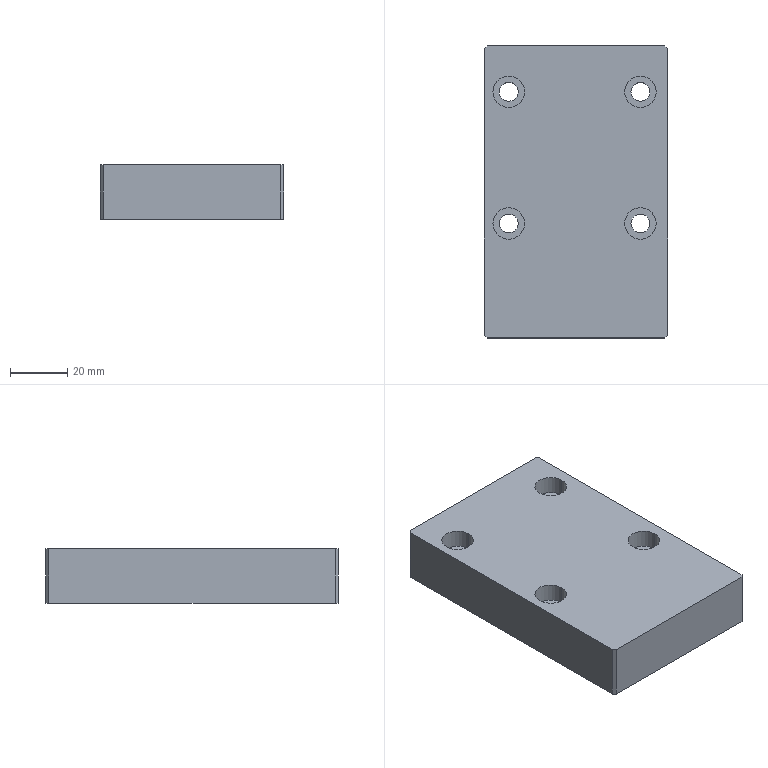Part | SolidWorks | features HoleWzd 4, Chamfer 2, Cut 1, Extrusion 1, ICE 1 | 1 solid | 50 faces | box 64 x 102 x 19 mm | volume 119355 mm3 | cylinder 26 | plane 14 | cone 10 | commonest cylinder face diameters 3.3 x10 6.6 x8 11 x8
STEP:
#1=CARTESIAN_POINT('',(-25.928,-4.723,12.6));
#2=VERTEX_POINT('',#1);
#3=CARTESIAN_POINT('',(-14.928,-4.723,12.6));
#4=VERTEX_POINT('',#3);
#5=CARTESIAN_POINT('',(-20.428,-4.723,12.6));
#6=DIRECTION('',(0.,0.,1.));
#7=DIRECTION('',(1.,0.,0.));
#8=AXIS2_PLACEMENT_3D('',#5,#6,#7);
#9=CIRCLE('',#8,5.5);
#10=EDGE_CURVE('',#2,#4,#9,.T.);
#11=ORIENTED_EDGE('',*,*,#10,.F.);
#12=CARTESIAN_POINT('',(-25.928,-4.723,19.));
#13=VERTEX_POINT('',#12);
#14=CARTESIAN_POINT('',(-25.928,-4.723,19.));
#15=DIRECTION('',(0.,0.,1.));
#16=VECTOR('',#15,1000.);
#17=LINE('',#14,#16);
#18=EDGE_CURVE('',#2,#13,#17,.T.);
#19=ORIENTED_EDGE('',*,*,#18,.T.);
#20=CARTESIAN_POINT('',(-14.928,-4.723,19.));
#21=VERTEX_POINT('',#20);
#22=CARTESIAN_POINT('',(-20.428,-4.723,19.));
#23=DIRECTION('',(0.,0.,1.));
#24=DIRECTION('',(1.,0.,0.));
#25=AXIS2_PLACEMENT_3D('',#22,#23,#24);
#26=CIRCLE('',#25,5.5);
#27=EDGE_CURVE('',#13,#21,#26,.T.);
#28=ORIENTED_EDGE('',*,*,#27,.T.);
#29=CARTESIAN_POINT('',(-14.928,-4.723,19.));
#30=DIRECTION('',(0.,0.,1.));
#31=VECTOR('',#30,1000.);
#32=LINE('',#29,#31);
#33=EDGE_CURVE('',#4,#21,#32,.T.);
#34=ORIENTED_EDGE('',*,*,#33,.F.);
#35=EDGE_LOOP('',(#11,#19,#28,#34));
#36=FACE_OUTER_BOUND('',#35,.T.);
#37=CARTESIAN_POINT('',(-20.428,-4.723,19.));
#38=DIRECTION('',(0.,0.,1.));
#39=DIRECTION('',(1.,0.,0.));
#40=AXIS2_PLACEMENT_3D('',#37,#38,#39);
#41=CYLINDRICAL_SURFACE('',#40,5.5);
#42=ADVANCED_FACE('',(#36),#41,.F.);
#43=CARTESIAN_POINT('',(-23.728,-4.723,0.));
#44=VERTEX_POINT('',#43);
#45=CARTESIAN_POINT('',(-17.128,-4.723,0.));
#46=VERTEX_POINT('',#45);
#47=CARTESIAN_POINT('',(-20.428,-4.723,0.));
#48=DIRECTION('',(0.,0.,1.));
#49=DIRECTION('',(1.,0.,0.));
#50=AXIS2_PLACEMENT_3D('',#47,#48,#49);
#51=CIRCLE('',#50,3.3);
#52=EDGE_CURVE('',#44,#46,#51,.T.);
#53=ORIENTED_EDGE('',*,*,#52,.F.);
#54=CARTESIAN_POINT('',(-23.728,-4.723,12.6));
#55=VERTEX_POINT('',#54);
#56=CARTESIAN_POINT('',(-23.728,-4.723,19.));
#57=DIRECTION('',(0.,0.,1.));
#58=VECTOR('',#57,1000.);
#59=LINE('',#56,#58);
#60=EDGE_CURVE('',#44,#55,#59,.T.);
#61=ORIENTED_EDGE('',*,*,#60,.T.);
#62=CARTESIAN_POINT('',(-17.128,-4.723,12.6));
#63=VERTEX_POINT('',#62);
#64=CARTESIAN_POINT('',(-20.428,-4.723,12.6));
#65=DIRECTION('',(0.,0.,1.));
#66=DIRECTION('',(1.,0.,0.));
#67=AXIS2_PLACEMENT_3D('',#64,#65,#66);
#68=CIRCLE('',#67,3.3);
#69=EDGE_CURVE('',#55,#63,#68,.T.);
#70=ORIENTED_EDGE('',*,*,#69,.T.);
#71=CARTESIAN_POINT('',(-17.128,-4.723,19.));
#72=DIRECTION('',(0.,0.,1.));
#73=VECTOR('',#72,1000.);
#74=LINE('',#71,#73);
#75=EDGE_CURVE('',#46,#63,#74,.T.);
#76=ORIENTED_EDGE('',*,*,#75,.F.);
#77=EDGE_LOOP('',(#53,#61,#70,#76));
#78=FACE_OUTER_BOUND('',#77,.T.);
#79=CARTESIAN_POINT('',(-20.428,-4.723,19.));
#80=DIRECTION('',(0.,0.,1.));
#81=DIRECTION('',(1.,0.,0.));
#82=AXIS2_PLACEMENT_3D('',#79,#80,#81);
#83=CYLINDRICAL_SURFACE('',#82,3.3);
#84=ADVANCED_FACE('',(#78),#83,.F.);
#85=CARTESIAN_POINT('',(20.072,-4.723,12.6));
#86=VERTEX_POINT('',#85);
#87=CARTESIAN_POINT('',(31.072,-4.723,12.6));
#88=VERTEX_POINT('',#87);
#89=CARTESIAN_POINT('',(25.572,-4.723,12.6));
#90=DIRECTION('',(0.,0.,1.));
#91=DIRECTION('',(1.,0.,0.));
#92=AXIS2_PLACEMENT_3D('',#89,#90,#91);
#93=CIRCLE('',#92,5.5);
#94=EDGE_CURVE('',#86,#88,#93,.T.);
#95=ORIENTED_EDGE('',*,*,#94,.F.);
#96=CARTESIAN_POINT('',(20.072,-4.723,19.));
#97=VERTEX_POINT('',#96);
#98=CARTESIAN_POINT('',(20.072,-4.723,19.));
#99=DIRECTION('',(0.,0.,1.));
#100=VECTOR('',#99,1000.);
#101=LINE('',#98,#100);
#102=EDGE_CURVE('',#86,#97,#101,.T.);
#103=ORIENTED_EDGE('',*,*,#102,.T.);
#104=CARTESIAN_POINT('',(31.072,-4.723,19.));
#105=VERTEX_POINT('',#104);
#106=CARTESIAN_POINT('',(25.572,-4.723,19.));
#107=DIRECTION('',(0.,0.,1.));
#108=DIRECTION('',(1.,0.,0.));
#109=AXIS2_PLACEMENT_3D('',#106,#107,#108);
#110=CIRCLE('',#109,5.5);
#111=EDGE_CURVE('',#97,#105,#110,.T.);
#112=ORIENTED_EDGE('',*,*,#111,.T.);
#113=CARTESIAN_POINT('',(31.072,-4.723,19.));
#114=DIRECTION('',(0.,0.,1.));
#115=VECTOR('',#114,1000.);
#116=LINE('',#113,#115);
#117=EDGE_CURVE('',#88,#105,#116,.T.);
#118=ORIENTED_EDGE('',*,*,#117,.F.);
#119=EDGE_LOOP('',(#95,#103,#112,#118));
#120=FACE_OUTER_BOUND('',#119,.T.);
#121=CARTESIAN_POINT('',(25.572,-4.723,19.));
#122=DIRECTION('',(0.,0.,1.));
#123=DIRECTION('',(1.,0.,0.));
#124=AXIS2_PLACEMENT_3D('',#121,#122,#123);
#125=CYLINDRICAL_SURFACE('',#124,5.5);
#126=ADVANCED_FACE('',(#120),#125,.F.);
#127=CARTESIAN_POINT('',(22.272,-4.723,0.));
#128=VERTEX_POINT('',#127);
#129=CARTESIAN_POINT('',(28.872,-4.723,0.));
#130=VERTEX_POINT('',#129);
#131=CARTESIAN_POINT('',(25.572,-4.723,0.));
#132=DIRECTION('',(0.,0.,1.));
#133=DIRECTION('',(1.,0.,0.));
#134=AXIS2_PLACEMENT_3D('',#131,#132,#133);
#135=CIRCLE('',#134,3.3);
#136=EDGE_CURVE('',#128,#130,#135,.T.);
#137=ORIENTED_EDGE('',*,*,#136,.F.);
#138=CARTESIAN_POINT('',(22.272,-4.723,12.6));
#139=VERTEX_POINT('',#138);
#140=CARTESIAN_POINT('',(22.272,-4.723,19.));
#141=DIRECTION('',(0.,0.,1.));
#142=VECTOR('',#141,1000.);
#143=LINE('',#140,#142);
#144=EDGE_CURVE('',#128,#139,#143,.T.);
#145=ORIENTED_EDGE('',*,*,#144,.T.);
#146=CARTESIAN_POINT('',(28.872,-4.723,12.6));
#147=VERTEX_POINT('',#146);
#148=CARTESIAN_POINT('',(25.572,-4.723,12.6));
#149=DIRECTION('',(0.,0.,1.));
#150=DIRECTION('',(1.,0.,0.));
#151=AXIS2_PLACEMENT_3D('',#148,#149,#150);
#152=CIRCLE('',#151,3.3);
#153=EDGE_CURVE('',#139,#147,#152,.T.);
#154=ORIENTED_EDGE('',*,*,#153,.T.);
#155=CARTESIAN_POINT('',(28.872,-4.723,19.));
#156=DIRECTION('',(0.,0.,1.));
#157=VECTOR('',#156,1000.);
#158=LINE('',#155,#157);
#159=EDGE_CURVE('',#130,#147,#158,.T.);
#160=ORIENTED_EDGE('',*,*,#159,.F.);
#161=EDGE_LOOP('',(#137,#145,#154,#160));
#162=FACE_OUTER_BOUND('',#161,.T.);
#163=CARTESIAN_POINT('',(25.572,-4.723,19.));
#164=DIRECTION('',(0.,0.,1.));
#165=DIRECTION('',(1.,0.,0.));
#166=AXIS2_PLACEMENT_3D('',#163,#164,#165);
#167=CYLINDRICAL_SURFACE('',#166,3.3);
#168=ADVANCED_FACE('',(#162),#167,.F.);
#169=CARTESIAN_POINT('',(20.072,-50.703,12.6));
#170=VERTEX_POINT('',#169);
#171=CARTESIAN_POINT('',(31.072,-50.703,12.6));
#172=VERTEX_POINT('',#171);
#173=CARTESIAN_POINT('',(25.572,-50.703,12.6));
#174=DIRECTION('',(0.,0.,1.));
#175=DIRECTION('',(1.,0.,0.));
#176=AXIS2_PLACEMENT_3D('',#173,#174,#175);
#177=CIRCLE('',#176,5.5);
#178=EDGE_CURVE('',#170,#172,#177,.T.);
#179=ORIENTED_EDGE('',*,*,#178,.F.);
#180=CARTESIAN_POINT('',(20.072,-50.703,19.));
#181=VERTEX_POINT('',#180);
#182=CARTESIAN_POINT('',(20.072,-50.703,19.));
#183=DIRECTION('',(0.,0.,1.));
#184=VECTOR('',#183,1000.);
#185=LINE('',#182,#184);
#186=EDGE_CURVE('',#170,#181,#185,.T.);
#187=ORIENTED_EDGE('',*,*,#186,.T.);
#188=CARTESIAN_POINT('',(31.072,-50.703,19.));
#189=VERTEX_POINT('',#188);
#190=CARTESIAN_POINT('',(25.572,-50.703,19.));
#191=DIRECTION('',(0.,0.,1.));
#192=DIRECTION('',(1.,0.,0.));
#193=AXIS2_PLACEMENT_3D('',#190,#191,#192);
#194=CIRCLE('',#193,5.5);
#195=EDGE_CURVE('',#181,#189,#194,.T.);
#196=ORIENTED_EDGE('',*,*,#195,.T.);
#197=CARTESIAN_POINT('',(31.072,-50.703,19.));
#198=DIRECTION('',(0.,0.,1.));
#199=VECTOR('',#198,1000.);
#200=LINE('',#197,#199);
#201=EDGE_CURVE('',#172,#189,#200,.T.);
#202=ORIENTED_EDGE('',*,*,#201,.F.);
#203=EDGE_LOOP('',(#179,#187,#196,#202));
#204=FACE_OUTER_BOUND('',#203,.T.);
#205=CARTESIAN_POINT('',(25.572,-50.703,19.));
#206=DIRECTION('',(0.,0.,1.));
#207=DIRECTION('',(1.,0.,0.));
#208=AXIS2_PLACEMENT_3D('',#205,#206,#207);
#209=CYLINDRICAL_SURFACE('',#208,5.5);
#210=ADVANCED_FACE('',(#204),#209,.F.);
#211=CARTESIAN_POINT('',(22.272,-50.703,0.));
#212=VERTEX_POINT('',#211);
#213=CARTESIAN_POINT('',(28.872,-50.703,0.));
#214=VERTEX_POINT('',#213);
#215=CARTESIAN_POINT('',(25.572,-50.703,0.));
#216=DIRECTION('',(0.,0.,1.));
#217=DIRECTION('',(1.,0.,0.));
#218=AXIS2_PLACEMENT_3D('',#215,#216,#217);
#219=CIRCLE('',#218,3.3);
#220=EDGE_CURVE('',#212,#214,#219,.T.);
#221=ORIENTED_EDGE('',*,*,#220,.F.);
#222=CARTESIAN_POINT('',(22.272,-50.703,12.6));
#223=VERTEX_POINT('',#222);
#224=CARTESIAN_POINT('',(22.272,-50.703,19.));
#225=DIRECTION('',(0.,0.,1.));
#226=VECTOR('',#225,1000.);
#227=LINE('',#224,#226);
#228=EDGE_CURVE('',#212,#223,#227,.T.);
#229=ORIENTED_EDGE('',*,*,#228,.T.);
#230=CARTESIAN_POINT('',(28.872,-50.703,12.6));
#231=VERTEX_POINT('',#230);
#232=CARTESIAN_POINT('',(25.572,-50.703,12.6));
#233=DIRECTION('',(0.,0.,1.));
#234=DIRECTION('',(1.,0.,0.));
#235=AXIS2_PLACEMENT_3D('',#232,#233,#234);
#236=CIRCLE('',#235,3.3);
#237=EDGE_CURVE('',#223,#231,#236,.T.);
#238=ORIENTED_EDGE('',*,*,#237,.T.);
#239=CARTESIAN_POINT('',(28.872,-50.703,19.));
#240=DIRECTION('',(0.,0.,1.));
#241=VECTOR('',#240,1000.);
#242=LINE('',#239,#241);
#243=EDGE_CURVE('',#214,#231,#242,.T.);
#244=ORIENTED_EDGE('',*,*,#243,.F.);
#245=EDGE_LOOP('',(#221,#229,#238,#244));
#246=FACE_OUTER_BOUND('',#245,.T.);
#247=CARTESIAN_POINT('',(25.572,-50.703,19.));
#248=DIRECTION('',(0.,0.,1.));
#249=DIRECTION('',(1.,0.,0.));
#250=AXIS2_PLACEMENT_3D('',#247,#248,#249);
#251=CYLINDRICAL_SURFACE('',#250,3.3);
#252=ADVANCED_FACE('',(#246),#251,.F.);
#253=CARTESIAN_POINT('',(-25.928,-50.723,12.6));
#254=VERTEX_POINT('',#253);
#255=CARTESIAN_POINT('',(-14.928,-50.723,12.6));
#256=VERTEX_POINT('',#255);
#257=CARTESIAN_POINT('',(-20.428,-50.723,12.6));
#258=DIRECTION('',(0.,0.,1.));
#259=DIRECTION('',(1.,0.,0.));
#260=AXIS2_PLACEMENT_3D('',#257,#258,#259);
#261=CIRCLE('',#260,5.5);
#262=EDGE_CURVE('',#254,#256,#261,.T.);
#263=ORIENTED_EDGE('',*,*,#262,.F.);
#264=CARTESIAN_POINT('',(-25.928,-50.723,19.));
#265=VERTEX_POINT('',#264);
#266=CARTESIAN_POINT('',(-25.928,-50.723,19.));
#267=DIRECTION('',(0.,0.,1.));
#268=VECTOR('',#267,1000.);
#269=LINE('',#266,#268);
#270=EDGE_CURVE('',#254,#265,#269,.T.);
#271=ORIENTED_EDGE('',*,*,#270,.T.);
#272=CARTESIAN_POINT('',(-14.928,-50.723,19.));
#273=VERTEX_POINT('',#272);
#274=CARTESIAN_POINT('',(-20.428,-50.723,19.));
#275=DIRECTION('',(0.,0.,1.));
#276=DIRECTION('',(1.,0.,0.));
#277=AXIS2_PLACEMENT_3D('',#274,#275,#276);
#278=CIRCLE('',#277,5.5);
#279=EDGE_CURVE('',#265,#273,#278,.T.);
#280=ORIENTED_EDGE('',*,*,#279,.T.);
#281=CARTESIAN_POINT('',(-14.928,-50.723,19.));
#282=DIRECTION('',(0.,0.,1.));
#283=VECTOR('',#282,1000.);
#284=LINE('',#281,#283);
#285=EDGE_CURVE('',#256,#273,#284,.T.);
#286=ORIENTED_EDGE('',*,*,#285,.F.);
#287=EDGE_LOOP('',(#263,#271,#280,#286));
#288=FACE_OUTER_BOUND('',#287,.T.);
#289=CARTESIAN_POINT('',(-20.428,-50.723,19.));
#290=DIRECTION('',(0.,0.,1.));
#291=DIRECTION('',(1.,0.,0.));
#292=AXIS2_PLACEMENT_3D('',#289,#290,#291);
#293=CYLINDRICAL_SURFACE('',#292,5.5);
#294=ADVANCED_FACE('',(#288),#293,.F.);
#295=CARTESIAN_POINT('',(-23.728,-50.723,0.));
#296=VERTEX_POINT('',#295);
#297=CARTESIAN_POINT('',(-17.128,-50.723,0.));
#298=VERTEX_POINT('',#297);
#299=CARTESIAN_POINT('',(-20.428,-50.723,0.));
#300=DIRECTION('',(0.,0.,1.));
#301=DIRECTION('',(1.,0.,0.));
#302=AXIS2_PLACEMENT_3D('',#299,#300,#301);
#303=CIRCLE('',#302,3.3);
#304=EDGE_CURVE('',#296,#298,#303,.T.);
#305=ORIENTED_EDGE('',*,*,#304,.F.);
#306=CARTESIAN_POINT('',(-23.728,-50.723,12.6));
#307=VERTEX_POINT('',#306);
#308=CARTESIAN_POINT('',(-23.728,-50.723,19.));
#309=DIRECTION('',(0.,0.,1.));
#310=VECTOR('',#309,1000.);
#311=LINE('',#308,#310);
#312=EDGE_CURVE('',#296,#307,#311,.T.);
#313=ORIENTED_EDGE('',*,*,#312,.T.);
#314=CARTESIAN_POINT('',(-17.128,-50.723,12.6));
#315=VERTEX_POINT('',#314);
#316=CARTESIAN_POINT('',(-20.428,-50.723,12.6));
#317=DIRECTION('',(0.,0.,1.));
#318=DIRECTION('',(1.,0.,0.));
#319=AXIS2_PLACEMENT_3D('',#316,#317,#318);
#320=CIRCLE('',#319,3.3);
#321=EDGE_CURVE('',#307,#315,#320,.T.);
#322=ORIENTED_EDGE('',*,*,#321,.T.);
#323=CARTESIAN_POINT('',(-17.128,-50.723,19.));
#324=DIRECTION('',(0.,0.,1.));
#325=VECTOR('',#324,1000.);
#326=LINE('',#323,#325);
#327=EDGE_CURVE('',#298,#315,#326,.T.);
#328=ORIENTED_EDGE('',*,*,#327,.F.);
#329=EDGE_LOOP('',(#305,#313,#322,#328));
#330=FACE_OUTER_BOUND('',#329,.T.);
#331=CARTESIAN_POINT('',(-20.428,-50.723,19.));
#332=DIRECTION('',(0.,0.,1.));
#333=DIRECTION('',(1.,0.,0.));
#334=AXIS2_PLACEMENT_3D('',#331,#332,#333);
#335=CYLINDRICAL_SURFACE('',#334,3.3);
#336=ADVANCED_FACE('',(#330),#335,.F.);
#337=CARTESIAN_POINT('',(14.722,7.277,10.1));
#338=VERTEX_POINT('',#337);
#339=CARTESIAN_POINT('',(11.422,7.277,10.1));
#340=VERTEX_POINT('',#339);
#341=CARTESIAN_POINT('',(13.072,7.277,10.1));
#342=DIRECTION('',(0.,0.,-1.));
#343=DIRECTION('',(-1.,0.,0.));
#344=AXIS2_PLACEMENT_3D('',#341,#342,#343);
#345=CIRCLE('',#344,1.65);
#346=EDGE_CURVE('',#338,#340,#345,.T.);
#347=ORIENTED_EDGE('',*,*,#346,.F.);
#348=CARTESIAN_POINT('',(14.722,7.277,0.));
#349=VERTEX_POINT('',#348);
#350=CARTESIAN_POINT('',(14.722,7.277,0.));
#351=DIRECTION('',(0.,0.,-1.));
#352=VECTOR('',#351,1000.);
#353=LINE('',#350,#352);
#354=EDGE_CURVE('',#338,#349,#353,.T.);
#355=ORIENTED_EDGE('',*,*,#354,.T.);
#356=CARTESIAN_POINT('',(11.422,7.277,0.));
#357=VERTEX_POINT('',#356);
#358=CARTESIAN_POINT('',(13.072,7.277,0.));
#359=DIRECTION('',(0.,0.,-1.));
#360=DIRECTION('',(-1.,0.,0.));
#361=AXIS2_PLACEMENT_3D('',#358,#359,#360);
#362=CIRCLE('',#361,1.65);
#363=EDGE_CURVE('',#349,#357,#362,.T.);
#364=ORIENTED_EDGE('',*,*,#363,.T.);
#365=CARTESIAN_POINT('',(11.422,7.277,0.));
#366=DIRECTION('',(0.,0.,-1.));
#367=VECTOR('',#366,1000.);
#368=LINE('',#365,#367);
#369=EDGE_CURVE('',#340,#357,#368,.T.);
#370=ORIENTED_EDGE('',*,*,#369,.F.);
#371=EDGE_LOOP('',(#347,#355,#364,#370));
#372=FACE_OUTER_BOUND('',#371,.T.);
#373=CARTESIAN_POINT('',(13.072,7.277,0.));
#374=DIRECTION('',(0.,0.,-1.));
#375=DIRECTION('',(-1.,0.,0.));
#376=AXIS2_PLACEMENT_3D('',#373,#374,#375);
#377=CYLINDRICAL_SURFACE('',#376,1.65);
#378=ADVANCED_FACE('',(#372),#377,.F.);
#379=CARTESIAN_POINT('',(13.072,7.277,11.091));
#380=VERTEX_POINT('',#379);
#381=CARTESIAN_POINT('',(11.422,7.277,10.1));
#382=DIRECTION('',(-0.8572,0.,-0.515));
#383=VECTOR('',#382,1000.);
#384=LINE('',#381,#383);
#385=EDGE_CURVE('',#380,#340,#384,.T.);
#386=ORIENTED_EDGE('',*,*,#385,.F.);
#387=CARTESIAN_POINT('',(14.722,7.277,10.1));
#388=DIRECTION('',(0.8572,0.,-0.515));
#389=VECTOR('',#388,1000.);
#390=LINE('',#387,#389);
#391=EDGE_CURVE('',#380,#338,#390,.T.);
#392=ORIENTED_EDGE('',*,*,#391,.T.);
#393=ORIENTED_EDGE('',*,*,#346,.T.);
#394=EDGE_LOOP('',(#386,#392,#393));
#395=FACE_OUTER_BOUND('',#394,.T.);
#396=CARTESIAN_POINT('',(13.072,7.277,10.1));
#397=DIRECTION('',(0.,0.,-1.));
#398=DIRECTION('',(-1.,0.,0.));
#399=AXIS2_PLACEMENT_3D('',#396,#397,#398);
#400=CONICAL_SURFACE('',#399,1.65,1.03);
#401=ADVANCED_FACE('',(#395),#400,.F.);
#402=CARTESIAN_POINT('',(-5.278,7.277,10.1));
#403=VERTEX_POINT('',#402);
#404=CARTESIAN_POINT('',(-8.578,7.277,10.1));
#405=VERTEX_POINT('',#404);
#406=CARTESIAN_POINT('',(-6.928,7.277,10.1));
#407=DIRECTION('',(0.,0.,-1.));
#408=DIRECTION('',(-1.,0.,0.));
#409=AXIS2_PLACEMENT_3D('',#406,#407,#408);
#410=CIRCLE('',#409,1.65);
#411=EDGE_CURVE('',#403,#405,#410,.T.);
#412=ORIENTED_EDGE('',*,*,#411,.F.);
#413=CARTESIAN_POINT('',(-5.278,7.277,0.));
#414=VERTEX_POINT('',#413);
#415=CARTESIAN_POINT('',(-5.278,7.277,0.));
#416=DIRECTION('',(0.,0.,-1.));
#417=VECTOR('',#416,1000.);
#418=LINE('',#415,#417);
#419=EDGE_CURVE('',#403,#414,#418,.T.);
#420=ORIENTED_EDGE('',*,*,#419,.T.);
#421=CARTESIAN_POINT('',(-8.578,7.277,0.));
#422=VERTEX_POINT('',#421);
#423=CARTESIAN_POINT('',(-6.928,7.277,0.));
#424=DIRECTION('',(0.,0.,-1.));
#425=DIRECTION('',(-1.,0.,0.));
#426=AXIS2_PLACEMENT_3D('',#423,#424,#425);
#427=CIRCLE('',#426,1.65);
#428=EDGE_CURVE('',#414,#422,#427,.T.);
#429=ORIENTED_EDGE('',*,*,#428,.T.);
#430=CARTESIAN_POINT('',(-8.578,7.277,0.));
#431=DIRECTION('',(0.,0.,-1.));
#432=VECTOR('',#431,1000.);
#433=LINE('',#430,#432);
#434=EDGE_CURVE('',#405,#422,#433,.T.);
#435=ORIENTED_EDGE('',*,*,#434,.F.);
#436=EDGE_LOOP('',(#412,#420,#429,#435));
#437=FACE_OUTER_BOUND('',#436,.T.);
#438=CARTESIAN_POINT('',(-6.928,7.277,0.));
#439=DIRECTION('',(0.,0.,-1.));
#440=DIRECTION('',(-1.,0.,0.));
#441=AXIS2_PLACEMENT_3D('',#438,#439,#440);
#442=CYLINDRICAL_SURFACE('',#441,1.65);
#443=ADVANCED_FACE('',(#437),#442,.F.);
#444=CARTESIAN_POINT('',(-6.928,7.277,11.091));
#445=VERTEX_POINT('',#444);
#446=CARTESIAN_POINT('',(-8.578,7.277,10.1));
#447=DIRECTION('',(-0.8572,0.,-0.515));
#448=VECTOR('',#447,1000.);
#449=LINE('',#446,#448);
#450=EDGE_CURVE('',#445,#405,#449,.T.);
#451=ORIENTED_EDGE('',*,*,#450,.F.);
#452=CARTESIAN_POINT('',(-5.278,7.277,10.1));
#453=DIRECTION('',(0.8572,0.,-0.515));
#454=VECTOR('',#453,1000.);
#455=LINE('',#452,#454);
#456=EDGE_CURVE('',#445,#403,#455,.T.);
#457=ORIENTED_EDGE('',*,*,#456,.T.);
#458=ORIENTED_EDGE('',*,*,#411,.T.);
#459=EDGE_LOOP('',(#451,#457,#458));
#460=FACE_OUTER_BOUND('',#459,.T.);
#461=CARTESIAN_POINT('',(-6.928,7.277,10.1));
#462=DIRECTION('',(0.,0.,-1.));
#463=DIRECTION('',(-1.,0.,0.));
#464=AXIS2_PLACEMENT_3D('',#461,#462,#463);
#465=CONICAL_SURFACE('',#464,1.65,1.03);
#466=ADVANCED_FACE('',(#460),#465,.F.);
#467=CARTESIAN_POINT('',(4.722,2.277,11.5));
#468=VERTEX_POINT('',#467);
#469=CARTESIAN_POINT('',(1.422,2.277,11.5));
#470=VERTEX_POINT('',#469);
#471=CARTESIAN_POINT('',(3.072,2.277,11.5));
#472=DIRECTION('',(0.,0.,-1.));
#473=DIRECTION('',(-1.,0.,0.));
#474=AXIS2_PLACEMENT_3D('',#471,#472,#473);
#475=CIRCLE('',#474,1.65);
#476=EDGE_CURVE('',#468,#470,#475,.T.);
#477=ORIENTED_EDGE('',*,*,#476,.F.);
#478=CARTESIAN_POINT('',(4.722,2.277,0.));
#479=VERTEX_POINT('',#478);
#480=CARTESIAN_POINT('',(4.722,2.277,0.));
#481=DIRECTION('',(0.,0.,-1.));
#482=VECTOR('',#481,1000.);
#483=LINE('',#480,#482);
#484=EDGE_CURVE('',#468,#479,#483,.T.);
#485=ORIENTED_EDGE('',*,*,#484,.T.);
#486=CARTESIAN_POINT('',(1.422,2.277,0.));
#487=VERTEX_POINT('',#486);
#488=CARTESIAN_POINT('',(3.072,2.277,0.));
#489=DIRECTION('',(0.,0.,-1.));
#490=DIRECTION('',(-1.,0.,0.));
#491=AXIS2_PLACEMENT_3D('',#488,#489,#490);
#492=CIRCLE('',#491,1.65);
#493=EDGE_CURVE('',#479,#487,#492,.T.);
#494=ORIENTED_EDGE('',*,*,#493,.T.);
#495=CARTESIAN_POINT('',(1.422,2.277,0.));
#496=DIRECTION('',(0.,0.,-1.));
#497=VECTOR('',#496,1000.);
#498=LINE('',#495,#497);
#499=EDGE_CURVE('',#470,#487,#498,.T.);
#500=ORIENTED_EDGE('',*,*,#499,.F.);
#501=EDGE_LOOP('',(#477,#485,#494,#500));
#502=FACE_OUTER_BOUND('',#501,.T.);
#503=CARTESIAN_POINT('',(3.072,2.277,0.));
#504=DIRECTION('',(0.,0.,-1.));
#505=DIRECTION('',(-1.,0.,0.));
#506=AXIS2_PLACEMENT_3D('',#503,#504,#505);
#507=CYLINDRICAL_SURFACE('',#506,1.65);
#508=ADVANCED_FACE('',(#502),#507,.F.);
#509=CARTESIAN_POINT('',(3.072,2.277,12.491));
#510=VERTEX_POINT('',#509);
#511=CARTESIAN_POINT('',(1.422,2.277,11.5));
#512=DIRECTION('',(-0.8572,0.,-0.515));
#513=VECTOR('',#512,1000.);
#514=LINE('',#511,#513);
#515=EDGE_CURVE('',#510,#470,#514,.T.);
#516=ORIENTED_EDGE('',*,*,#515,.F.);
#517=CARTESIAN_POINT('',(4.722,2.277,11.5));
#518=DIRECTION('',(0.8572,0.,-0.515));
#519=VECTOR('',#518,1000.);
#520=LINE('',#517,#519);
#521=EDGE_CURVE('',#510,#468,#520,.T.);
#522=ORIENTED_EDGE('',*,*,#521,.T.);
#523=ORIENTED_EDGE('',*,*,#476,.T.);
#524=EDGE_LOOP('',(#516,#522,#523));
#525=FACE_OUTER_BOUND('',#524,.T.);
#526=CARTESIAN_POINT('',(3.072,2.277,11.5));
#527=DIRECTION('',(0.,0.,-1.));
#528=DIRECTION('',(-1.,0.,0.));
#529=AXIS2_PLACEMENT_3D('',#526,#527,#528);
#530=CONICAL_SURFACE('',#529,1.65,1.03);
#531=ADVANCED_FACE('',(#525),#530,.F.);
#532=CARTESIAN_POINT('',(4.722,-26.723,11.5));
#533=VERTEX_POINT('',#532);
#534=CARTESIAN_POINT('',(1.422,-26.723,11.5));
#535=VERTEX_POINT('',#534);
#536=CARTESIAN_POINT('',(3.072,-26.723,11.5));
#537=DIRECTION('',(0.,0.,-1.));
#538=DIRECTION('',(-1.,0.,0.));
#539=AXIS2_PLACEMENT_3D('',#536,#537,#538);
#540=CIRCLE('',#539,1.65);
#541=EDGE_CURVE('',#533,#535,#540,.T.);
#542=ORIENTED_EDGE('',*,*,#541,.F.);
#543=CARTESIAN_POINT('',(4.722,-26.723,0.));
#544=VERTEX_POINT('',#543);
#545=CARTESIAN_POINT('',(4.722,-26.723,0.));
#546=DIRECTION('',(0.,0.,-1.));
#547=VECTOR('',#546,1000.);
#548=LINE('',#545,#547);
#549=EDGE_CURVE('',#533,#544,#548,.T.);
#550=ORIENTED_EDGE('',*,*,#549,.T.);
#551=CARTESIAN_POINT('',(1.422,-26.723,0.));
#552=VERTEX_POINT('',#551);
#553=CARTESIAN_POINT('',(3.072,-26.723,0.));
#554=DIRECTION('',(0.,0.,-1.));
#555=DIRECTION('',(-1.,0.,0.));
#556=AXIS2_PLACEMENT_3D('',#553,#554,#555);
#557=CIRCLE('',#556,1.65);
#558=EDGE_CURVE('',#544,#552,#557,.T.);
#559=ORIENTED_EDGE('',*,*,#558,.T.);
#560=CARTESIAN_POINT('',(1.422,-26.723,0.));
#561=DIRECTION('',(0.,0.,-1.));
#562=VECTOR('',#561,1000.);
#563=LINE('',#560,#562);
#564=EDGE_CURVE('',#535,#552,#563,.T.);
#565=ORIENTED_EDGE('',*,*,#564,.F.);
#566=EDGE_LOOP('',(#542,#550,#559,#565));
#567=FACE_OUTER_BOUND('',#566,.T.);
#568=CARTESIAN_POINT('',(3.072,-26.723,0.));
#569=DIRECTION('',(0.,0.,-1.));
#570=DIRECTION('',(-1.,0.,0.));
#571=AXIS2_PLACEMENT_3D('',#568,#569,#570);
#572=CYLINDRICAL_SURFACE('',#571,1.65);
#573=ADVANCED_FACE('',(#567),#572,.F.);
#574=CARTESIAN_POINT('',(3.072,-26.723,12.491));
#575=VERTEX_POINT('',#574);
#576=CARTESIAN_POINT('',(1.422,-26.723,11.5));
#577=DIRECTION('',(-0.8572,0.,-0.515));
#578=VECTOR('',#577,1000.);
#579=LINE('',#576,#578);
#580=EDGE_CURVE('',#575,#535,#579,.T.);
#581=ORIENTED_EDGE('',*,*,#580,.F.);
#582=CARTESIAN_POINT('',(4.722,-26.723,11.5));
#583=DIRECTION('',(0.8572,0.,-0.515));
#584=VECTOR('',#583,1000.);
#585=LINE('',#582,#584);
#586=EDGE_CURVE('',#575,#533,#585,.T.);
#587=ORIENTED_EDGE('',*,*,#586,.T.);
#588=ORIENTED_EDGE('',*,*,#541,.T.);
#589=EDGE_LOOP('',(#581,#587,#588));
#590=FACE_OUTER_BOUND('',#589,.T.);
#591=CARTESIAN_POINT('',(3.072,-26.723,11.5));
#592=DIRECTION('',(0.,0.,-1.));
#593=DIRECTION('',(-1.,0.,0.));
#594=AXIS2_PLACEMENT_3D('',#591,#592,#593);
#595=CONICAL_SURFACE('',#594,1.65,1.03);
#596=ADVANCED_FACE('',(#590),#595,.F.);
#597=CARTESIAN_POINT('',(4.722,-65.723,11.5));
#598=VERTEX_POINT('',#597);
#599=CARTESIAN_POINT('',(1.422,-65.723,11.5));
#600=VERTEX_POINT('',#599);
#601=CARTESIAN_POINT('',(3.072,-65.723,11.5));
#602=DIRECTION('',(0.,0.,-1.));
#603=DIRECTION('',(-1.,0.,0.));
#604=AXIS2_PLACEMENT_3D('',#601,#602,#603);
#605=CIRCLE('',#604,1.65);
#606=EDGE_CURVE('',#598,#600,#605,.T.);
#607=ORIENTED_EDGE('',*,*,#606,.F.);
#608=CARTESIAN_POINT('',(4.722,-65.723,0.));
#609=VERTEX_POINT('',#608);
#610=CARTESIAN_POINT('',(4.722,-65.723,0.));
#611=DIRECTION('',(0.,0.,-1.));
#612=VECTOR('',#611,1000.);
#613=LINE('',#610,#612);
#614=EDGE_CURVE('',#598,#609,#613,.T.);
#615=ORIENTED_EDGE('',*,*,#614,.T.);
#616=CARTESIAN_POINT('',(1.422,-65.723,0.));
#617=VERTEX_POINT('',#616);
#618=CARTESIAN_POINT('',(3.072,-65.723,0.));
#619=DIRECTION('',(0.,0.,-1.));
#620=DIRECTION('',(-1.,0.,0.));
#621=AXIS2_PLACEMENT_3D('',#618,#619,#620);
#622=CIRCLE('',#621,1.65);
#623=EDGE_CURVE('',#609,#617,#622,.T.);
#624=ORIENTED_EDGE('',*,*,#623,.T.);
#625=CARTESIAN_POINT('',(1.422,-65.723,0.));
#626=DIRECTION('',(0.,0.,-1.));
#627=VECTOR('',#626,1000.);
#628=LINE('',#625,#627);
#629=EDGE_CURVE('',#600,#617,#628,.T.);
#630=ORIENTED_EDGE('',*,*,#629,.F.);
#631=EDGE_LOOP('',(#607,#615,#624,#630));
#632=FACE_OUTER_BOUND('',#631,.T.);
#633=CARTESIAN_POINT('',(3.072,-65.723,0.));
#634=DIRECTION('',(0.,0.,-1.));
#635=DIRECTION('',(-1.,0.,0.));
#636=AXIS2_PLACEMENT_3D('',#633,#634,#635);
#637=CYLINDRICAL_SURFACE('',#636,1.65);
#638=ADVANCED_FACE('',(#632),#637,.F.);
#639=CARTESIAN_POINT('',(3.072,-65.723,12.491));
#640=VERTEX_POINT('',#639);
#641=CARTESIAN_POINT('',(1.422,-65.723,11.5));
#642=DIRECTION('',(-0.8572,0.,-0.515));
#643=VECTOR('',#642,1000.);
#644=LINE('',#641,#643);
#645=EDGE_CURVE('',#640,#600,#644,.T.);
#646=ORIENTED_EDGE('',*,*,#645,.F.);
#647=CARTESIAN_POINT('',(4.722,-65.723,11.5));
#648=DIRECTION('',(0.8572,0.,-0.515));
#649=VECTOR('',#648,1000.);
#650=LINE('',#647,#649);
#651=EDGE_CURVE('',#640,#598,#650,.T.);
#652=ORIENTED_EDGE('',*,*,#651,.T.);
#653=ORIENTED_EDGE('',*,*,#606,.T.);
#654=EDGE_LOOP('',(#646,#652,#653));
#655=FACE_OUTER_BOUND('',#654,.T.);
#656=CARTESIAN_POINT('',(3.072,-65.723,11.5));
#657=DIRECTION('',(0.,0.,-1.));
#658=DIRECTION('',(-1.,0.,0.));
#659=AXIS2_PLACEMENT_3D('',#656,#657,#658);
#660=CONICAL_SURFACE('',#659,1.65,1.03);
#661=ADVANCED_FACE('',(#655),#660,.F.);
#662=CARTESIAN_POINT('',(-27.928,-90.723,0.));
#663=VERTEX_POINT('',#662);
#664=CARTESIAN_POINT('',(34.072,-90.723,0.));
#665=VERTEX_POINT('',#664);
#666=CARTESIAN_POINT('',(-18.928,-90.723,0.));
#667=DIRECTION('',(1.,0.,0.));
#668=VECTOR('',#667,1000.);
#669=LINE('',#666,#668);
#670=EDGE_CURVE('',#663,#665,#669,.T.);
#671=ORIENTED_EDGE('',*,*,#670,.T.);
#672=CARTESIAN_POINT('',(34.072,-90.723,19.));
#673=VERTEX_POINT('',#672);
#674=CARTESIAN_POINT('',(34.072,-90.723,19.));
#675=DIRECTION('',(0.,0.,1.));
#676=VECTOR('',#675,1000.);
#677=LINE('',#674,#676);
#678=EDGE_CURVE('',#665,#673,#677,.T.);
#679=ORIENTED_EDGE('',*,*,#678,.T.);
#680=CARTESIAN_POINT('',(-27.928,-90.723,19.));
#681=VERTEX_POINT('',#680);
#682=CARTESIAN_POINT('',(-18.928,-90.723,19.));
#683=DIRECTION('',(1.,0.,0.));
#684=VECTOR('',#683,1000.);
#685=LINE('',#682,#684);
#686=EDGE_CURVE('',#681,#673,#685,.T.);
#687=ORIENTED_EDGE('',*,*,#686,.F.);
#688=CARTESIAN_POINT('',(-27.928,-90.723,0.));
#689=DIRECTION('',(0.,0.,-1.));
#690=VECTOR('',#689,1000.);
#691=LINE('',#688,#690);
#692=EDGE_CURVE('',#681,#663,#691,.T.);
#693=ORIENTED_EDGE('',*,*,#692,.T.);
#694=EDGE_LOOP('',(#671,#679,#687,#693));
#695=FACE_OUTER_BOUND('',#694,.T.);
#696=CARTESIAN_POINT('',(-18.928,-90.723,19.));
#697=DIRECTION('',(0.,1.,0.));
#698=DIRECTION('',(0.,0.,1.));
#699=AXIS2_PLACEMENT_3D('',#696,#697,#698);
#700=PLANE('',#699);
#701=ADVANCED_FACE('',(#695),#700,.F.);
#702=CARTESIAN_POINT('',(-20.428,-4.723,19.));
#703=DIRECTION('',(0.,0.,1.));
#704=DIRECTION('',(1.,0.,0.));
#705=AXIS2_PLACEMENT_3D('',#702,#703,#704);
#706=CIRCLE('',#705,5.5);
#707=EDGE_CURVE('',#21,#13,#706,.T.);
#708=ORIENTED_EDGE('',*,*,#707,.F.);
#709=ORIENTED_EDGE('',*,*,#27,.F.);
#710=EDGE_LOOP('',(#708,#709));
#711=FACE_BOUND('',#710,.T.);
#712=CARTESIAN_POINT('',(25.572,-4.723,19.));
#713=DIRECTION('',(0.,0.,1.));
#714=DIRECTION('',(1.,0.,0.));
#715=AXIS2_PLACEMENT_3D('',#712,#713,#714);
#716=CIRCLE('',#715,5.5);
#717=EDGE_CURVE('',#105,#97,#716,.T.);
#718=ORIENTED_EDGE('',*,*,#717,.F.);
#719=ORIENTED_EDGE('',*,*,#111,.F.);
#720=EDGE_LOOP('',(#718,#719));
#721=FACE_BOUND('',#720,.T.);
#722=CARTESIAN_POINT('',(25.572,-50.703,19.));
#723=DIRECTION('',(0.,0.,1.));
#724=DIRECTION('',(1.,0.,0.));
#725=AXIS2_PLACEMENT_3D('',#722,#723,#724);
#726=CIRCLE('',#725,5.5);
#727=EDGE_CURVE('',#189,#181,#726,.T.);
#728=ORIENTED_EDGE('',*,*,#727,.F.);
#729=ORIENTED_EDGE('',*,*,#195,.F.);
#730=EDGE_LOOP('',(#728,#729));
#731=FACE_BOUND('',#730,.T.);
#732=CARTESIAN_POINT('',(-20.428,-50.723,19.));
#733=DIRECTION('',(0.,0.,1.));
#734=DIRECTION('',(1.,0.,0.));
#735=AXIS2_PLACEMENT_3D('',#732,#733,#734);
#736=CIRCLE('',#735,5.5);
#737=EDGE_CURVE('',#273,#265,#736,.T.);
#738=ORIENTED_EDGE('',*,*,#737,.F.);
#739=ORIENTED_EDGE('',*,*,#279,.F.);
#740=EDGE_LOOP('',(#738,#739));
#741=FACE_BOUND('',#740,.T.);
#742=ORIENTED_EDGE('',*,*,#686,.T.);
#743=CARTESIAN_POINT('',(35.072,-89.723,19.));
#744=VERTEX_POINT('',#743);
#745=CARTESIAN_POINT('',(62.398,-62.398,19.));
#746=DIRECTION('',(0.7071,0.7071,0.));
#747=VECTOR('',#746,1000.);
#748=LINE('',#745,#747);
#749=EDGE_CURVE('',#673,#744,#748,.T.);
#750=ORIENTED_EDGE('',*,*,#749,.T.);
#751=CARTESIAN_POINT('',(35.072,10.277,19.));
#752=VERTEX_POINT('',#751);
#753=CARTESIAN_POINT('',(35.072,11.277,19.));
#754=DIRECTION('',(0.,1.,0.));
#755=VECTOR('',#754,1000.);
#756=LINE('',#753,#755);
#757=EDGE_CURVE('',#744,#752,#756,.T.);
#758=ORIENTED_EDGE('',*,*,#757,.T.);
#759=CARTESIAN_POINT('',(34.072,11.277,19.));
#760=VERTEX_POINT('',#759);
#761=CARTESIAN_POINT('',(22.675,22.675,19.));
#762=DIRECTION('',(-0.7071,0.7071,0.));
#763=VECTOR('',#762,1000.);
#764=LINE('',#761,#763);
#765=EDGE_CURVE('',#752,#760,#764,.T.);
#766=ORIENTED_EDGE('',*,*,#765,.T.);
#767=CARTESIAN_POINT('',(-27.928,11.277,19.));
#768=VERTEX_POINT('',#767);
#769=CARTESIAN_POINT('',(-18.928,11.277,19.));
#770=DIRECTION('',(1.,0.,0.));
#771=VECTOR('',#770,1000.);
#772=LINE('',#769,#771);
#773=EDGE_CURVE('',#768,#760,#772,.T.);
#774=ORIENTED_EDGE('',*,*,#773,.F.);
#775=CARTESIAN_POINT('',(-28.928,10.277,19.));
#776=VERTEX_POINT('',#775);
#777=CARTESIAN_POINT('',(-19.602,19.602,19.));
#778=DIRECTION('',(-0.7071,-0.7071,0.));
#779=VECTOR('',#778,1000.);
#780=LINE('',#777,#779);
#781=EDGE_CURVE('',#768,#776,#780,.T.);
#782=ORIENTED_EDGE('',*,*,#781,.T.);
#783=CARTESIAN_POINT('',(-28.928,-89.723,19.));
#784=VERTEX_POINT('',#783);
#785=CARTESIAN_POINT('',(-28.928,11.277,19.));
#786=DIRECTION('',(0.,-1.,0.));
#787=VECTOR('',#786,1000.);
#788=LINE('',#785,#787);
#789=EDGE_CURVE('',#776,#784,#788,.T.);
#790=ORIENTED_EDGE('',*,*,#789,.T.);
#791=CARTESIAN_POINT('',(-59.325,-59.325,19.));
#792=DIRECTION('',(0.7071,-0.7071,0.));
#793=VECTOR('',#792,1000.);
#794=LINE('',#791,#793);
#795=EDGE_CURVE('',#784,#681,#794,.T.);
#796=ORIENTED_EDGE('',*,*,#795,.T.);
#797=EDGE_LOOP('',(#742,#750,#758,#766,#774,#782,#790,#796));
#798=FACE_OUTER_BOUND('',#797,.T.);
#799=CARTESIAN_POINT('',(0.,0.,19.));
#800=DIRECTION('',(0.,0.,1.));
#801=DIRECTION('',(1.,0.,0.));
#802=AXIS2_PLACEMENT_3D('',#799,#800,#801);
#803=PLANE('',#802);
#804=ADVANCED_FACE('',(#711,#721,#731,#741,#798),#803,.T.);
#805=CARTESIAN_POINT('',(-20.428,-4.723,0.));
#806=DIRECTION('',(0.,0.,1.));
#807=DIRECTION('',(1.,0.,0.));
#808=AXIS2_PLACEMENT_3D('',#805,#806,#807);
#809=CIRCLE('',#808,3.3);
#810=EDGE_CURVE('',#46,#44,#809,.T.);
#811=ORIENTED_EDGE('',*,*,#810,.T.);
#812=ORIENTED_EDGE('',*,*,#52,.T.);
#813=EDGE_LOOP('',(#811,#812));
#814=FACE_BOUND('',#813,.T.);
#815=CARTESIAN_POINT('',(25.572,-4.723,0.));
#816=DIRECTION('',(0.,0.,1.));
#817=DIRECTION('',(1.,0.,0.));
#818=AXIS2_PLACEMENT_3D('',#815,#816,#817);
#819=CIRCLE('',#818,3.3);
#820=EDGE_CURVE('',#130,#128,#819,.T.);
#821=ORIENTED_EDGE('',*,*,#820,.T.);
#822=ORIENTED_EDGE('',*,*,#136,.T.);
#823=EDGE_LOOP('',(#821,#822));
#824=FACE_BOUND('',#823,.T.);
#825=CARTESIAN_POINT('',(25.572,-50.703,0.));
#826=DIRECTION('',(0.,0.,1.));
#827=DIRECTION('',(1.,0.,0.));
#828=AXIS2_PLACEMENT_3D('',#825,#826,#827);
#829=CIRCLE('',#828,3.3);
#830=EDGE_CURVE('',#214,#212,#829,.T.);
#831=ORIENTED_EDGE('',*,*,#830,.T.);
#832=ORIENTED_EDGE('',*,*,#220,.T.);
#833=EDGE_LOOP('',(#831,#832));
#834=FACE_BOUND('',#833,.T.);
#835=CARTESIAN_POINT('',(-20.428,-50.723,0.));
#836=DIRECTION('',(0.,0.,1.));
#837=DIRECTION('',(1.,0.,0.));
#838=AXIS2_PLACEMENT_3D('',#835,#836,#837);
#839=CIRCLE('',#838,3.3);
#840=EDGE_CURVE('',#298,#296,#839,.T.);
#841=ORIENTED_EDGE('',*,*,#840,.T.);
#842=ORIENTED_EDGE('',*,*,#304,.T.);
#843=EDGE_LOOP('',(#841,#842));
#844=FACE_BOUND('',#843,.T.);
#845=CARTESIAN_POINT('',(13.072,7.277,0.));
#846=DIRECTION('',(0.,0.,-1.));
#847=DIRECTION('',(-1.,0.,0.));
#848=AXIS2_PLACEMENT_3D('',#845,#846,#847);
#849=CIRCLE('',#848,1.65);
#850=EDGE_CURVE('',#357,#349,#849,.T.);
#851=ORIENTED_EDGE('',*,*,#850,.F.);
#852=ORIENTED_EDGE('',*,*,#363,.F.);
#853=EDGE_LOOP('',(#851,#852));
#854=FACE_BOUND('',#853,.T.);
#855=CARTESIAN_POINT('',(-6.928,7.277,0.));
#856=DIRECTION('',(0.,0.,-1.));
#857=DIRECTION('',(-1.,0.,0.));
#858=AXIS2_PLACEMENT_3D('',#855,#856,#857);
#859=CIRCLE('',#858,1.65);
#860=EDGE_CURVE('',#422,#414,#859,.T.);
#861=ORIENTED_EDGE('',*,*,#860,.F.);
#862=ORIENTED_EDGE('',*,*,#428,.F.);
#863=EDGE_LOOP('',(#861,#862));
#864=FACE_BOUND('',#863,.T.);
#865=CARTESIAN_POINT('',(3.072,2.277,0.));
#866=DIRECTION('',(0.,0.,-1.));
#867=DIRECTION('',(-1.,0.,0.));
#868=AXIS2_PLACEMENT_3D('',#865,#866,#867);
#869=CIRCLE('',#868,1.65);
#870=EDGE_CURVE('',#487,#479,#869,.T.);
#871=ORIENTED_EDGE('',*,*,#870,.F.);
#872=ORIENTED_EDGE('',*,*,#493,.F.);
#873=EDGE_LOOP('',(#871,#872));
#874=FACE_BOUND('',#873,.T.);
#875=CARTESIAN_POINT('',(3.072,-26.723,0.));
#876=DIRECTION('',(0.,0.,-1.));
#877=DIRECTION('',(-1.,0.,0.));
#878=AXIS2_PLACEMENT_3D('',#875,#876,#877);
#879=CIRCLE('',#878,1.65);
#880=EDGE_CURVE('',#552,#544,#879,.T.);
#881=ORIENTED_EDGE('',*,*,#880,.F.);
#882=ORIENTED_EDGE('',*,*,#558,.F.);
#883=EDGE_LOOP('',(#881,#882));
#884=FACE_BOUND('',#883,.T.);
#885=CARTESIAN_POINT('',(3.072,-65.723,0.));
#886=DIRECTION('',(0.,0.,-1.));
#887=DIRECTION('',(-1.,0.,0.));
#888=AXIS2_PLACEMENT_3D('',#885,#886,#887);
#889=CIRCLE('',#888,1.65);
#890=EDGE_CURVE('',#617,#609,#889,.T.);
#891=ORIENTED_EDGE('',*,*,#890,.F.);
#892=ORIENTED_EDGE('',*,*,#623,.F.);
#893=EDGE_LOOP('',(#891,#892));
#894=FACE_BOUND('',#893,.T.);
#895=CARTESIAN_POINT('',(35.072,-89.723,0.));
#896=VERTEX_POINT('',#895);
#897=CARTESIAN_POINT('',(35.072,10.277,0.));
#898=VERTEX_POINT('',#897);
#899=CARTESIAN_POINT('',(35.072,11.277,0.));
#900=DIRECTION('',(0.,1.,0.));
#901=VECTOR('',#900,1000.);
#902=LINE('',#899,#901);
#903=EDGE_CURVE('',#896,#898,#902,.T.);
#904=ORIENTED_EDGE('',*,*,#903,.F.);
#905=CARTESIAN_POINT('',(34.072,-90.723,0.));
#906=DIRECTION('',(-0.7071,-0.7071,0.));
#907=VECTOR('',#906,1000.);
#908=LINE('',#905,#907);
#909=EDGE_CURVE('',#896,#665,#908,.T.);
#910=ORIENTED_EDGE('',*,*,#909,.T.);
#911=ORIENTED_EDGE('',*,*,#670,.F.);
#912=CARTESIAN_POINT('',(-28.928,-89.723,0.));
#913=VERTEX_POINT('',#912);
#914=CARTESIAN_POINT('',(-28.928,-89.723,0.));
#915=DIRECTION('',(-0.7071,0.7071,0.));
#916=VECTOR('',#915,1000.);
#917=LINE('',#914,#916);
#918=EDGE_CURVE('',#663,#913,#917,.T.);
#919=ORIENTED_EDGE('',*,*,#918,.T.);
#920=CARTESIAN_POINT('',(-28.928,10.277,0.));
#921=VERTEX_POINT('',#920);
#922=CARTESIAN_POINT('',(-28.928,11.277,0.));
#923=DIRECTION('',(0.,-1.,0.));
#924=VECTOR('',#923,1000.);
#925=LINE('',#922,#924);
#926=EDGE_CURVE('',#921,#913,#925,.T.);
#927=ORIENTED_EDGE('',*,*,#926,.F.);
#928=CARTESIAN_POINT('',(-27.928,11.277,0.));
#929=VERTEX_POINT('',#928);
#930=CARTESIAN_POINT('',(-27.928,11.277,0.));
#931=DIRECTION('',(0.7071,0.7071,0.));
#932=VECTOR('',#931,1000.);
#933=LINE('',#930,#932);
#934=EDGE_CURVE('',#921,#929,#933,.T.);
#935=ORIENTED_EDGE('',*,*,#934,.T.);
#936=CARTESIAN_POINT('',(34.072,11.277,0.));
#937=VERTEX_POINT('',#936);
#938=CARTESIAN_POINT('',(-18.928,11.277,0.));
#939=DIRECTION('',(1.,0.,0.));
#940=VECTOR('',#939,1000.);
#941=LINE('',#938,#940);
#942=EDGE_CURVE('',#929,#937,#941,.T.);
#943=ORIENTED_EDGE('',*,*,#942,.T.);
#944=CARTESIAN_POINT('',(35.072,10.277,0.));
#945=DIRECTION('',(0.7071,-0.7071,0.));
#946=VECTOR('',#945,1000.);
#947=LINE('',#944,#946);
#948=EDGE_CURVE('',#937,#898,#947,.T.);
#949=ORIENTED_EDGE('',*,*,#948,.T.);
#950=EDGE_LOOP('',(#904,#910,#911,#919,#927,#935,#943,#949));
#951=FACE_OUTER_BOUND('',#950,.T.);
#952=CARTESIAN_POINT('',(0.,0.,0.));
#953=DIRECTION('',(0.,0.,1.));
#954=DIRECTION('',(1.,0.,0.));
#955=AXIS2_PLACEMENT_3D('',#952,#953,#954);
#956=PLANE('',#955);
#957=ADVANCED_FACE('',(#814,#824,#834,#844,#854,#864,#874,#884,#894,#951),#956,.F.);
#958=ORIENTED_EDGE('',*,*,#651,.F.);
#959=ORIENTED_EDGE('',*,*,#645,.T.);
#960=CARTESIAN_POINT('',(3.072,-65.723,11.5));
#961=DIRECTION('',(0.,0.,-1.));
#962=DIRECTION('',(-1.,0.,0.));
#963=AXIS2_PLACEMENT_3D('',#960,#961,#962);
#964=CIRCLE('',#963,1.65);
#965=EDGE_CURVE('',#600,#598,#964,.T.);
#966=ORIENTED_EDGE('',*,*,#965,.T.);
#967=EDGE_LOOP('',(#958,#959,#966));
#968=FACE_OUTER_BOUND('',#967,.T.);
#969=CARTESIAN_POINT('',(3.072,-65.723,11.5));
#970=DIRECTION('',(0.,0.,-1.));
#971=DIRECTION('',(-1.,0.,0.));
#972=AXIS2_PLACEMENT_3D('',#969,#970,#971);
#973=CONICAL_SURFACE('',#972,1.65,1.03);
#974=ADVANCED_FACE('',(#968),#973,.F.);
#975=ORIENTED_EDGE('',*,*,#614,.F.);
#976=ORIENTED_EDGE('',*,*,#965,.F.);
#977=ORIENTED_EDGE('',*,*,#629,.T.);
#978=ORIENTED_EDGE('',*,*,#890,.T.);
#979=EDGE_LOOP('',(#975,#976,#977,#978));
#980=FACE_OUTER_BOUND('',#979,.T.);
#981=CARTESIAN_POINT('',(3.072,-65.723,0.));
#982=DIRECTION('',(0.,0.,-1.));
#983=DIRECTION('',(-1.,0.,0.));
#984=AXIS2_PLACEMENT_3D('',#981,#982,#983);
#985=CYLINDRICAL_SURFACE('',#984,1.65);
#986=ADVANCED_FACE('',(#980),#985,.F.);
#987=ORIENTED_EDGE('',*,*,#586,.F.);
#988=ORIENTED_EDGE('',*,*,#580,.T.);
#989=CARTESIAN_POINT('',(3.072,-26.723,11.5));
#990=DIRECTION('',(0.,0.,-1.));
#991=DIRECTION('',(-1.,0.,0.));
#992=AXIS2_PLACEMENT_3D('',#989,#990,#991);
#993=CIRCLE('',#992,1.65);
#994=EDGE_CURVE('',#535,#533,#993,.T.);
#995=ORIENTED_EDGE('',*,*,#994,.T.);
#996=EDGE_LOOP('',(#987,#988,#995));
#997=FACE_OUTER_BOUND('',#996,.T.);
#998=CARTESIAN_POINT('',(3.072,-26.723,11.5));
#999=DIRECTION('',(0.,0.,-1.));
#1000=DIRECTION('',(-1.,0.,0.));
#1001=AXIS2_PLACEMENT_3D('',#998,#999,#1000);
#1002=CONICAL_SURFACE('',#1001,1.65,1.03);
#1003=ADVANCED_FACE('',(#997),#1002,.F.);
#1004=ORIENTED_EDGE('',*,*,#549,.F.);
#1005=ORIENTED_EDGE('',*,*,#994,.F.);
#1006=ORIENTED_EDGE('',*,*,#564,.T.);
#1007=ORIENTED_EDGE('',*,*,#880,.T.);
#1008=EDGE_LOOP('',(#1004,#1005,#1006,#1007));
#1009=FACE_OUTER_BOUND('',#1008,.T.);
#1010=CARTESIAN_POINT('',(3.072,-26.723,0.));
#1011=DIRECTION('',(0.,0.,-1.));
#1012=DIRECTION('',(-1.,0.,0.));
#1013=AXIS2_PLACEMENT_3D('',#1010,#1011,#1012);
#1014=CYLINDRICAL_SURFACE('',#1013,1.65);
#1015=ADVANCED_FACE('',(#1009),#1014,.F.);
#1016=ORIENTED_EDGE('',*,*,#521,.F.);
#1017=ORIENTED_EDGE('',*,*,#515,.T.);
#1018=CARTESIAN_POINT('',(3.072,2.277,11.5));
#1019=DIRECTION('',(0.,0.,-1.));
#1020=DIRECTION('',(-1.,0.,0.));
#1021=AXIS2_PLACEMENT_3D('',#1018,#1019,#1020);
#1022=CIRCLE('',#1021,1.65);
#1023=EDGE_CURVE('',#470,#468,#1022,.T.);
#1024=ORIENTED_EDGE('',*,*,#1023,.T.);
#1025=EDGE_LOOP('',(#1016,#1017,#1024));
#1026=FACE_OUTER_BOUND('',#1025,.T.);
#1027=CARTESIAN_POINT('',(3.072,2.277,11.5));
#1028=DIRECTION('',(0.,0.,-1.));
#1029=DIRECTION('',(-1.,0.,0.));
#1030=AXIS2_PLACEMENT_3D('',#1027,#1028,#1029);
#1031=CONICAL_SURFACE('',#1030,1.65,1.03);
#1032=ADVANCED_FACE('',(#1026),#1031,.F.);
#1033=ORIENTED_EDGE('',*,*,#484,.F.);
#1034=ORIENTED_EDGE('',*,*,#1023,.F.);
#1035=ORIENTED_EDGE('',*,*,#499,.T.);
#1036=ORIENTED_EDGE('',*,*,#870,.T.);
#1037=EDGE_LOOP('',(#1033,#1034,#1035,#1036));
#1038=FACE_OUTER_BOUND('',#1037,.T.);
#1039=CARTESIAN_POINT('',(3.072,2.277,0.));
#1040=DIRECTION('',(0.,0.,-1.));
#1041=DIRECTION('',(-1.,0.,0.));
#1042=AXIS2_PLACEMENT_3D('',#1039,#1040,#1041);
#1043=CYLINDRICAL_SURFACE('',#1042,1.65);
#1044=ADVANCED_FACE('',(#1038),#1043,.F.);
#1045=ORIENTED_EDGE('',*,*,#773,.T.);
#1046=CARTESIAN_POINT('',(34.072,11.277,0.));
#1047=DIRECTION('',(0.,0.,-1.));
#1048=VECTOR('',#1047,1000.);
#1049=LINE('',#1046,#1048);
#1050=EDGE_CURVE('',#760,#937,#1049,.T.);
#1051=ORIENTED_EDGE('',*,*,#1050,.T.);
#1052=ORIENTED_EDGE('',*,*,#942,.F.);
#1053=CARTESIAN_POINT('',(-27.928,11.277,19.));
#1054=DIRECTION('',(0.,0.,1.));
#1055=VECTOR('',#1054,1000.);
#1056=LINE('',#1053,#1055);
#1057=EDGE_CURVE('',#929,#768,#1056,.T.);
#1058=ORIENTED_EDGE('',*,*,#1057,.T.);
#1059=EDGE_LOOP('',(#1045,#1051,#1052,#1058));
#1060=FACE_OUTER_BOUND('',#1059,.T.);
#1061=CARTESIAN_POINT('',(-18.928,11.277,0.));
#1062=DIRECTION('',(0.,-1.,0.));
#1063=DIRECTION('',(1.,0.,0.));
#1064=AXIS2_PLACEMENT_3D('',#1061,#1062,#1063);
#1065=PLANE('',#1064);
#1066=ADVANCED_FACE('',(#1060),#1065,.F.);
#1067=ORIENTED_EDGE('',*,*,#456,.F.);
#1068=ORIENTED_EDGE('',*,*,#450,.T.);
#1069=CARTESIAN_POINT('',(-6.928,7.277,10.1));
#1070=DIRECTION('',(0.,0.,-1.));
#1071=DIRECTION('',(-1.,0.,0.));
#1072=AXIS2_PLACEMENT_3D('',#1069,#1070,#1071);
#1073=CIRCLE('',#1072,1.65);
#1074=EDGE_CURVE('',#405,#403,#1073,.T.);
#1075=ORIENTED_EDGE('',*,*,#1074,.T.);
#1076=EDGE_LOOP('',(#1067,#1068,#1075));
#1077=FACE_OUTER_BOUND('',#1076,.T.);
#1078=CARTESIAN_POINT('',(-6.928,7.277,10.1));
#1079=DIRECTION('',(0.,0.,-1.));
#1080=DIRECTION('',(-1.,0.,0.));
#1081=AXIS2_PLACEMENT_3D('',#1078,#1079,#1080);
#1082=CONICAL_SURFACE('',#1081,1.65,1.03);
#1083=ADVANCED_FACE('',(#1077),#1082,.F.);
#1084=ORIENTED_EDGE('',*,*,#419,.F.);
#1085=ORIENTED_EDGE('',*,*,#1074,.F.);
#1086=ORIENTED_EDGE('',*,*,#434,.T.);
#1087=ORIENTED_EDGE('',*,*,#860,.T.);
#1088=EDGE_LOOP('',(#1084,#1085,#1086,#1087));
#1089=FACE_OUTER_BOUND('',#1088,.T.);
#1090=CARTESIAN_POINT('',(-6.928,7.277,0.));
#1091=DIRECTION('',(0.,0.,-1.));
#1092=DIRECTION('',(-1.,0.,0.));
#1093=AXIS2_PLACEMENT_3D('',#1090,#1091,#1092);
#1094=CYLINDRICAL_SURFACE('',#1093,1.65);
#1095=ADVANCED_FACE('',(#1089),#1094,.F.);
#1096=ORIENTED_EDGE('',*,*,#391,.F.);
#1097=ORIENTED_EDGE('',*,*,#385,.T.);
#1098=CARTESIAN_POINT('',(13.072,7.277,10.1));
#1099=DIRECTION('',(0.,0.,-1.));
#1100=DIRECTION('',(-1.,0.,0.));
#1101=AXIS2_PLACEMENT_3D('',#1098,#1099,#1100);
#1102=CIRCLE('',#1101,1.65);
#1103=EDGE_CURVE('',#340,#338,#1102,.T.);
#1104=ORIENTED_EDGE('',*,*,#1103,.T.);
#1105=EDGE_LOOP('',(#1096,#1097,#1104));
#1106=FACE_OUTER_BOUND('',#1105,.T.);
#1107=CARTESIAN_POINT('',(13.072,7.277,10.1));
#1108=DIRECTION('',(0.,0.,-1.));
#1109=DIRECTION('',(-1.,0.,0.));
#1110=AXIS2_PLACEMENT_3D('',#1107,#1108,#1109);
#1111=CONICAL_SURFACE('',#1110,1.65,1.03);
#1112=ADVANCED_FACE('',(#1106),#1111,.F.);
#1113=ORIENTED_EDGE('',*,*,#354,.F.);
#1114=ORIENTED_EDGE('',*,*,#1103,.F.);
#1115=ORIENTED_EDGE('',*,*,#369,.T.);
#1116=ORIENTED_EDGE('',*,*,#850,.T.);
#1117=EDGE_LOOP('',(#1113,#1114,#1115,#1116));
#1118=FACE_OUTER_BOUND('',#1117,.T.);
#1119=CARTESIAN_POINT('',(13.072,7.277,0.));
#1120=DIRECTION('',(0.,0.,-1.));
#1121=DIRECTION('',(-1.,0.,0.));
#1122=AXIS2_PLACEMENT_3D('',#1119,#1120,#1121);
#1123=CYLINDRICAL_SURFACE('',#1122,1.65);
#1124=ADVANCED_FACE('',(#1118),#1123,.F.);
#1125=ORIENTED_EDGE('',*,*,#926,.T.);
#1126=CARTESIAN_POINT('',(-28.928,-89.723,19.));
#1127=DIRECTION('',(0.,0.,1.));
#1128=VECTOR('',#1127,1000.);
#1129=LINE('',#1126,#1128);
#1130=EDGE_CURVE('',#913,#784,#1129,.T.);
#1131=ORIENTED_EDGE('',*,*,#1130,.T.);
#1132=ORIENTED_EDGE('',*,*,#789,.F.);
#1133=CARTESIAN_POINT('',(-28.928,10.277,0.));
#1134=DIRECTION('',(0.,0.,-1.));
#1135=VECTOR('',#1134,1000.);
#1136=LINE('',#1133,#1135);
#1137=EDGE_CURVE('',#776,#921,#1136,.T.);
#1138=ORIENTED_EDGE('',*,*,#1137,.T.);
#1139=EDGE_LOOP('',(#1125,#1131,#1132,#1138));
#1140=FACE_OUTER_BOUND('',#1139,.T.);
#1141=CARTESIAN_POINT('',(-28.928,11.277,0.));
#1142=DIRECTION('',(-1.,0.,0.));
#1143=DIRECTION('',(0.,-1.,0.));
#1144=AXIS2_PLACEMENT_3D('',#1141,#1142,#1143);
#1145=PLANE('',#1144);
#1146=ADVANCED_FACE('',(#1140),#1145,.T.);
#1147=ORIENTED_EDGE('',*,*,#757,.F.);
#1148=CARTESIAN_POINT('',(35.072,-89.723,0.));
#1149=DIRECTION('',(0.,0.,-1.));
#1150=VECTOR('',#1149,1000.);
#1151=LINE('',#1148,#1150);
#1152=EDGE_CURVE('',#744,#896,#1151,.T.);
#1153=ORIENTED_EDGE('',*,*,#1152,.T.);
#1154=ORIENTED_EDGE('',*,*,#903,.T.);
#1155=CARTESIAN_POINT('',(35.072,10.277,19.));
#1156=DIRECTION('',(0.,0.,1.));
#1157=VECTOR('',#1156,1000.);
#1158=LINE('',#1155,#1157);
#1159=EDGE_CURVE('',#898,#752,#1158,.T.);
#1160=ORIENTED_EDGE('',*,*,#1159,.T.);
#1161=EDGE_LOOP('',(#1147,#1153,#1154,#1160));
#1162=FACE_OUTER_BOUND('',#1161,.T.);
#1163=CARTESIAN_POINT('',(35.072,11.277,0.));
#1164=DIRECTION('',(1.,0.,0.));
#1165=DIRECTION('',(0.,1.,0.));
#1166=AXIS2_PLACEMENT_3D('',#1163,#1164,#1165);
#1167=PLANE('',#1166);
#1168=ADVANCED_FACE('',(#1162),#1167,.T.);
#1169=ORIENTED_EDGE('',*,*,#312,.F.);
#1170=ORIENTED_EDGE('',*,*,#840,.F.);
#1171=ORIENTED_EDGE('',*,*,#327,.T.);
#1172=CARTESIAN_POINT('',(-20.428,-50.723,12.6));
#1173=DIRECTION('',(0.,0.,1.));
#1174=DIRECTION('',(1.,0.,0.));
#1175=AXIS2_PLACEMENT_3D('',#1172,#1173,#1174);
#1176=CIRCLE('',#1175,3.3);
#1177=EDGE_CURVE('',#315,#307,#1176,.T.);
#1178=ORIENTED_EDGE('',*,*,#1177,.T.);
#1179=EDGE_LOOP('',(#1169,#1170,#1171,#1178));
#1180=FACE_OUTER_BOUND('',#1179,.T.);
#1181=CARTESIAN_POINT('',(-20.428,-50.723,19.));
#1182=DIRECTION('',(0.,0.,1.));
#1183=DIRECTION('',(1.,0.,0.));
#1184=AXIS2_PLACEMENT_3D('',#1181,#1182,#1183);
#1185=CYLINDRICAL_SURFACE('',#1184,3.3);
#1186=ADVANCED_FACE('',(#1180),#1185,.F.);
#1187=ORIENTED_EDGE('',*,*,#1177,.F.);
#1188=ORIENTED_EDGE('',*,*,#321,.F.);
#1189=EDGE_LOOP('',(#1187,#1188));
#1190=FACE_BOUND('',#1189,.T.);
#1191=CARTESIAN_POINT('',(-20.428,-50.723,12.6));
#1192=DIRECTION('',(0.,0.,1.));
#1193=DIRECTION('',(1.,0.,0.));
#1194=AXIS2_PLACEMENT_3D('',#1191,#1192,#1193);
#1195=CIRCLE('',#1194,5.5);
#1196=EDGE_CURVE('',#256,#254,#1195,.T.);
#1197=ORIENTED_EDGE('',*,*,#1196,.T.);
#1198=ORIENTED_EDGE('',*,*,#262,.T.);
#1199=EDGE_LOOP('',(#1197,#1198));
#1200=FACE_OUTER_BOUND('',#1199,.T.);
#1201=CARTESIAN_POINT('',(-17.128,-50.723,12.6));
#1202=DIRECTION('',(0.,0.,-1.));
#1203=DIRECTION('',(-1.,0.,0.));
#1204=AXIS2_PLACEMENT_3D('',#1201,#1202,#1203);
#1205=PLANE('',#1204);
#1206=ADVANCED_FACE('',(#1190,#1200),#1205,.F.);
#1207=ORIENTED_EDGE('',*,*,#270,.F.);
#1208=ORIENTED_EDGE('',*,*,#1196,.F.);
#1209=ORIENTED_EDGE('',*,*,#285,.T.);
#1210=ORIENTED_EDGE('',*,*,#737,.T.);
#1211=EDGE_LOOP('',(#1207,#1208,#1209,#1210));
#1212=FACE_OUTER_BOUND('',#1211,.T.);
#1213=CARTESIAN_POINT('',(-20.428,-50.723,19.));
#1214=DIRECTION('',(0.,0.,1.));
#1215=DIRECTION('',(1.,0.,0.));
#1216=AXIS2_PLACEMENT_3D('',#1213,#1214,#1215);
#1217=CYLINDRICAL_SURFACE('',#1216,5.5);
#1218=ADVANCED_FACE('',(#1212),#1217,.F.);
#1219=ORIENTED_EDGE('',*,*,#228,.F.);
#1220=ORIENTED_EDGE('',*,*,#830,.F.);
#1221=ORIENTED_EDGE('',*,*,#243,.T.);
#1222=CARTESIAN_POINT('',(25.572,-50.703,12.6));
#1223=DIRECTION('',(0.,0.,1.));
#1224=DIRECTION('',(1.,0.,0.));
#1225=AXIS2_PLACEMENT_3D('',#1222,#1223,#1224);
#1226=CIRCLE('',#1225,3.3);
#1227=EDGE_CURVE('',#231,#223,#1226,.T.);
#1228=ORIENTED_EDGE('',*,*,#1227,.T.);
#1229=EDGE_LOOP('',(#1219,#1220,#1221,#1228));
#1230=FACE_OUTER_BOUND('',#1229,.T.);
#1231=CARTESIAN_POINT('',(25.572,-50.703,19.));
#1232=DIRECTION('',(0.,0.,1.));
#1233=DIRECTION('',(1.,0.,0.));
#1234=AXIS2_PLACEMENT_3D('',#1231,#1232,#1233);
#1235=CYLINDRICAL_SURFACE('',#1234,3.3);
#1236=ADVANCED_FACE('',(#1230),#1235,.F.);
#1237=ORIENTED_EDGE('',*,*,#1227,.F.);
#1238=ORIENTED_EDGE('',*,*,#237,.F.);
#1239=EDGE_LOOP('',(#1237,#1238));
#1240=FACE_BOUND('',#1239,.T.);
#1241=CARTESIAN_POINT('',(25.572,-50.703,12.6));
#1242=DIRECTION('',(0.,0.,1.));
#1243=DIRECTION('',(1.,0.,0.));
#1244=AXIS2_PLACEMENT_3D('',#1241,#1242,#1243);
#1245=CIRCLE('',#1244,5.5);
#1246=EDGE_CURVE('',#172,#170,#1245,.T.);
#1247=ORIENTED_EDGE('',*,*,#1246,.T.);
#1248=ORIENTED_EDGE('',*,*,#178,.T.);
#1249=EDGE_LOOP('',(#1247,#1248));
#1250=FACE_OUTER_BOUND('',#1249,.T.);
#1251=CARTESIAN_POINT('',(28.872,-50.703,12.6));
#1252=DIRECTION('',(0.,0.,-1.));
#1253=DIRECTION('',(-1.,0.,0.));
#1254=AXIS2_PLACEMENT_3D('',#1251,#1252,#1253);
#1255=PLANE('',#1254);
#1256=ADVANCED_FACE('',(#1240,#1250),#1255,.F.);
#1257=ORIENTED_EDGE('',*,*,#186,.F.);
#1258=ORIENTED_EDGE('',*,*,#1246,.F.);
#1259=ORIENTED_EDGE('',*,*,#201,.T.);
#1260=ORIENTED_EDGE('',*,*,#727,.T.);
#1261=EDGE_LOOP('',(#1257,#1258,#1259,#1260));
#1262=FACE_OUTER_BOUND('',#1261,.T.);
#1263=CARTESIAN_POINT('',(25.572,-50.703,19.));
#1264=DIRECTION('',(0.,0.,1.));
#1265=DIRECTION('',(1.,0.,0.));
#1266=AXIS2_PLACEMENT_3D('',#1263,#1264,#1265);
#1267=CYLINDRICAL_SURFACE('',#1266,5.5);
#1268=ADVANCED_FACE('',(#1262),#1267,.F.);
#1269=ORIENTED_EDGE('',*,*,#144,.F.);
#1270=ORIENTED_EDGE('',*,*,#820,.F.);
#1271=ORIENTED_EDGE('',*,*,#159,.T.);
#1272=CARTESIAN_POINT('',(25.572,-4.723,12.6));
#1273=DIRECTION('',(0.,0.,1.));
#1274=DIRECTION('',(1.,0.,0.));
#1275=AXIS2_PLACEMENT_3D('',#1272,#1273,#1274);
#1276=CIRCLE('',#1275,3.3);
#1277=EDGE_CURVE('',#147,#139,#1276,.T.);
#1278=ORIENTED_EDGE('',*,*,#1277,.T.);
#1279=EDGE_LOOP('',(#1269,#1270,#1271,#1278));
#1280=FACE_OUTER_BOUND('',#1279,.T.);
#1281=CARTESIAN_POINT('',(25.572,-4.723,19.));
#1282=DIRECTION('',(0.,0.,1.));
#1283=DIRECTION('',(1.,0.,0.));
#1284=AXIS2_PLACEMENT_3D('',#1281,#1282,#1283);
#1285=CYLINDRICAL_SURFACE('',#1284,3.3);
#1286=ADVANCED_FACE('',(#1280),#1285,.F.);
#1287=ORIENTED_EDGE('',*,*,#1277,.F.);
#1288=ORIENTED_EDGE('',*,*,#153,.F.);
#1289=EDGE_LOOP('',(#1287,#1288));
#1290=FACE_BOUND('',#1289,.T.);
#1291=CARTESIAN_POINT('',(25.572,-4.723,12.6));
#1292=DIRECTION('',(0.,0.,1.));
#1293=DIRECTION('',(1.,0.,0.));
#1294=AXIS2_PLACEMENT_3D('',#1291,#1292,#1293);
#1295=CIRCLE('',#1294,5.5);
#1296=EDGE_CURVE('',#88,#86,#1295,.T.);
#1297=ORIENTED_EDGE('',*,*,#1296,.T.);
#1298=ORIENTED_EDGE('',*,*,#94,.T.);
#1299=EDGE_LOOP('',(#1297,#1298));
#1300=FACE_OUTER_BOUND('',#1299,.T.);
#1301=CARTESIAN_POINT('',(28.872,-4.723,12.6));
#1302=DIRECTION('',(0.,0.,-1.));
#1303=DIRECTION('',(-1.,0.,0.));
#1304=AXIS2_PLACEMENT_3D('',#1301,#1302,#1303);
#1305=PLANE('',#1304);
#1306=ADVANCED_FACE('',(#1290,#1300),#1305,.F.);
#1307=ORIENTED_EDGE('',*,*,#102,.F.);
#1308=ORIENTED_EDGE('',*,*,#1296,.F.);
#1309=ORIENTED_EDGE('',*,*,#117,.T.);
#1310=ORIENTED_EDGE('',*,*,#717,.T.);
#1311=EDGE_LOOP('',(#1307,#1308,#1309,#1310));
#1312=FACE_OUTER_BOUND('',#1311,.T.);
#1313=CARTESIAN_POINT('',(25.572,-4.723,19.));
#1314=DIRECTION('',(0.,0.,1.));
#1315=DIRECTION('',(1.,0.,0.));
#1316=AXIS2_PLACEMENT_3D('',#1313,#1314,#1315);
#1317=CYLINDRICAL_SURFACE('',#1316,5.5);
#1318=ADVANCED_FACE('',(#1312),#1317,.F.);
#1319=ORIENTED_EDGE('',*,*,#60,.F.);
#1320=ORIENTED_EDGE('',*,*,#810,.F.);
#1321=ORIENTED_EDGE('',*,*,#75,.T.);
#1322=CARTESIAN_POINT('',(-20.428,-4.723,12.6));
#1323=DIRECTION('',(0.,0.,1.));
#1324=DIRECTION('',(1.,0.,0.));
#1325=AXIS2_PLACEMENT_3D('',#1322,#1323,#1324);
#1326=CIRCLE('',#1325,3.3);
#1327=EDGE_CURVE('',#63,#55,#1326,.T.);
#1328=ORIENTED_EDGE('',*,*,#1327,.T.);
#1329=EDGE_LOOP('',(#1319,#1320,#1321,#1328));
#1330=FACE_OUTER_BOUND('',#1329,.T.);
#1331=CARTESIAN_POINT('',(-20.428,-4.723,19.));
#1332=DIRECTION('',(0.,0.,1.));
#1333=DIRECTION('',(1.,0.,0.));
#1334=AXIS2_PLACEMENT_3D('',#1331,#1332,#1333);
#1335=CYLINDRICAL_SURFACE('',#1334,3.3);
#1336=ADVANCED_FACE('',(#1330),#1335,.F.);
#1337=ORIENTED_EDGE('',*,*,#1327,.F.);
#1338=ORIENTED_EDGE('',*,*,#69,.F.);
#1339=EDGE_LOOP('',(#1337,#1338));
#1340=FACE_BOUND('',#1339,.T.);
#1341=CARTESIAN_POINT('',(-20.428,-4.723,12.6));
#1342=DIRECTION('',(0.,0.,1.));
#1343=DIRECTION('',(1.,0.,0.));
#1344=AXIS2_PLACEMENT_3D('',#1341,#1342,#1343);
#1345=CIRCLE('',#1344,5.5);
#1346=EDGE_CURVE('',#4,#2,#1345,.T.);
#1347=ORIENTED_EDGE('',*,*,#1346,.T.);
#1348=ORIENTED_EDGE('',*,*,#10,.T.);
#1349=EDGE_LOOP('',(#1347,#1348));
#1350=FACE_OUTER_BOUND('',#1349,.T.);
#1351=CARTESIAN_POINT('',(-17.128,-4.723,12.6));
#1352=DIRECTION('',(0.,0.,-1.));
#1353=DIRECTION('',(-1.,0.,0.));
#1354=AXIS2_PLACEMENT_3D('',#1351,#1352,#1353);
#1355=PLANE('',#1354);
#1356=ADVANCED_FACE('',(#1340,#1350),#1355,.F.);
#1357=ORIENTED_EDGE('',*,*,#18,.F.);
#1358=ORIENTED_EDGE('',*,*,#1346,.F.);
#1359=ORIENTED_EDGE('',*,*,#33,.T.);
#1360=ORIENTED_EDGE('',*,*,#707,.T.);
#1361=EDGE_LOOP('',(#1357,#1358,#1359,#1360));
#1362=FACE_OUTER_BOUND('',#1361,.T.);
#1363=CARTESIAN_POINT('',(-20.428,-4.723,19.));
#1364=DIRECTION('',(0.,0.,1.));
#1365=DIRECTION('',(1.,0.,0.));
#1366=AXIS2_PLACEMENT_3D('',#1363,#1364,#1365);
#1367=CYLINDRICAL_SURFACE('',#1366,5.5);
#1368=ADVANCED_FACE('',(#1362),#1367,.F.);
#1369=ORIENTED_EDGE('',*,*,#909,.F.);
#1370=ORIENTED_EDGE('',*,*,#1152,.F.);
#1371=ORIENTED_EDGE('',*,*,#749,.F.);
#1372=ORIENTED_EDGE('',*,*,#678,.F.);
#1373=EDGE_LOOP('',(#1369,#1370,#1371,#1372));
#1374=FACE_OUTER_BOUND('',#1373,.T.);
#1375=CARTESIAN_POINT('',(34.072,-90.723,19.));
#1376=DIRECTION('',(0.7071,-0.7071,0.));
#1377=DIRECTION('',(0.,0.,-1.));
#1378=AXIS2_PLACEMENT_3D('',#1375,#1376,#1377);
#1379=PLANE('',#1378);
#1380=ADVANCED_FACE('',(#1374),#1379,.T.);
#1381=ORIENTED_EDGE('',*,*,#918,.F.);
#1382=ORIENTED_EDGE('',*,*,#692,.F.);
#1383=ORIENTED_EDGE('',*,*,#795,.F.);
#1384=ORIENTED_EDGE('',*,*,#1130,.F.);
#1385=EDGE_LOOP('',(#1381,#1382,#1383,#1384));
#1386=FACE_OUTER_BOUND('',#1385,.T.);
#1387=CARTESIAN_POINT('',(-28.928,-89.723,0.));
#1388=DIRECTION('',(-0.7071,-0.7071,0.));
#1389=DIRECTION('',(0.,0.,-1.));
#1390=AXIS2_PLACEMENT_3D('',#1387,#1388,#1389);
#1391=PLANE('',#1390);
#1392=ADVANCED_FACE('',(#1386),#1391,.T.);
#1393=ORIENTED_EDGE('',*,*,#948,.F.);
#1394=ORIENTED_EDGE('',*,*,#1050,.F.);
#1395=ORIENTED_EDGE('',*,*,#765,.F.);
#1396=ORIENTED_EDGE('',*,*,#1159,.F.);
#1397=EDGE_LOOP('',(#1393,#1394,#1395,#1396));
#1398=FACE_OUTER_BOUND('',#1397,.T.);
#1399=CARTESIAN_POINT('',(35.072,10.277,0.));
#1400=DIRECTION('',(0.7071,0.7071,0.));
#1401=DIRECTION('',(0.,0.,-1.));
#1402=AXIS2_PLACEMENT_3D('',#1399,#1400,#1401);
#1403=PLANE('',#1402);
#1404=ADVANCED_FACE('',(#1398),#1403,.T.);
#1405=ORIENTED_EDGE('',*,*,#934,.F.);
#1406=ORIENTED_EDGE('',*,*,#1137,.F.);
#1407=ORIENTED_EDGE('',*,*,#781,.F.);
#1408=ORIENTED_EDGE('',*,*,#1057,.F.);
#1409=EDGE_LOOP('',(#1405,#1406,#1407,#1408));
#1410=FACE_OUTER_BOUND('',#1409,.T.);
#1411=CARTESIAN_POINT('',(-27.928,11.277,0.));
#1412=DIRECTION('',(-0.7071,0.7071,0.));
#1413=DIRECTION('',(0.,0.,-1.));
#1414=AXIS2_PLACEMENT_3D('',#1411,#1412,#1413);
#1415=PLANE('',#1414);
#1416=ADVANCED_FACE('',(#1410),#1415,.T.);
#1417=CLOSED_SHELL('',(#42,#84,#126,#168,#210,#252,#294,#336,#378,#401,#443,#466,#508,#531,#573,#596,#638,#661,#701,#804,#957,#974,#986,#1003,#1015,#1032,#1044,#1066,#1083,#1095,#1112,#1124,#1146,#1168,#1186,#1206,#1218,#1236,#1256,#1268,#1286,#1306,#1318,#1336,#1356,#1368,#1380,#1392,#1404,#1416));
#1418=MANIFOLD_SOLID_BREP('',#1417);
#1419=CARTESIAN_POINT('',(0.,0.,0.));
#1420=DIRECTION('',(0.,0.,1.));
#1421=DIRECTION('',(1.,0.,0.));
#1422=AXIS2_PLACEMENT_3D('',#1419,#1420,#1421);
#1423=(LENGTH_UNIT()NAMED_UNIT(*)SI_UNIT(.MILLI.,.METRE.));
#1424=UNCERTAINTY_MEASURE_WITH_UNIT(LENGTH_MEASURE(0.00001),#1423,'','');
#1425=(NAMED_UNIT(*)PLANE_ANGLE_UNIT()SI_UNIT($,.RADIAN.));
#1426=(NAMED_UNIT(*)SI_UNIT($,.STERADIAN.)SOLID_ANGLE_UNIT());
#1427=(GEOMETRIC_REPRESENTATION_CONTEXT(3)GLOBAL_UNCERTAINTY_ASSIGNED_CONTEXT((#1424))GLOBAL_UNIT_ASSIGNED_CONTEXT((#1423,#1425,#1426))REPRESENTATION_CONTEXT('',''));
#1428=ADVANCED_BREP_SHAPE_REPRESENTATION('',(#1418,#1422),#1427);